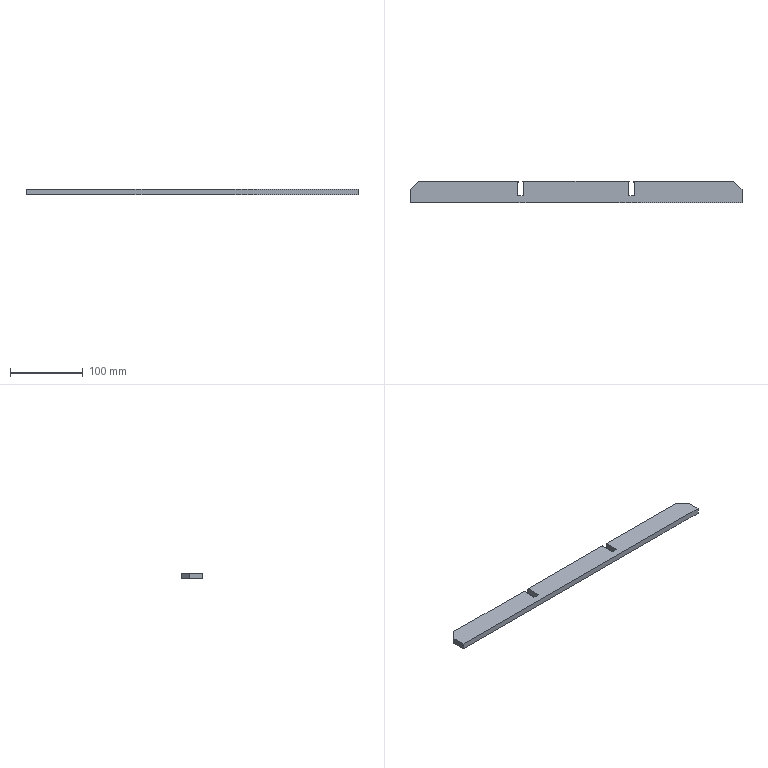Part | SolidWorks | features BaseBody 1 | 1 solid | 18 faces | box 455.8 x 30 x 8 mm | volume 104640 mm3 | plane 18
STEP:
#1=CARTESIAN_POINT('',(73.126,14.398,0.));
#2=VERTEX_POINT('',#1);
#3=CARTESIAN_POINT('',(73.412,15.,8.));
#4=VERTEX_POINT('',#3);
#5=CARTESIAN_POINT('',(73.126,14.398,0.));
#6=DIRECTION('',(0.0356,0.07493,0.9966));
#7=VECTOR('',#6,1000.);
#8=LINE('',#5,#7);
#9=EDGE_CURVE('',#2,#4,#8,.T.);
#10=ORIENTED_EDGE('',*,*,#9,.F.);
#11=CARTESIAN_POINT('',(-73.126,14.398,0.));
#12=VERTEX_POINT('',#11);
#13=CARTESIAN_POINT('',(0.,14.398,0.));
#14=DIRECTION('',(1.,0.,0.));
#15=VECTOR('',#14,1000.);
#16=LINE('',#13,#15);
#17=EDGE_CURVE('',#12,#2,#16,.T.);
#18=ORIENTED_EDGE('',*,*,#17,.F.);
#19=CARTESIAN_POINT('',(-73.412,15.,8.));
#20=VERTEX_POINT('',#19);
#21=CARTESIAN_POINT('',(-73.412,15.,8.));
#22=DIRECTION('',(0.0356,-0.07493,-0.9966));
#23=VECTOR('',#22,1000.);
#24=LINE('',#21,#23);
#25=EDGE_CURVE('',#20,#12,#24,.T.);
#26=ORIENTED_EDGE('',*,*,#25,.F.);
#27=CARTESIAN_POINT('',(0.,15.,8.));
#28=DIRECTION('',(-1.,0.,0.));
#29=VECTOR('',#28,1000.);
#30=LINE('',#27,#29);
#31=EDGE_CURVE('',#4,#20,#30,.T.);
#32=ORIENTED_EDGE('',*,*,#31,.F.);
#33=EDGE_LOOP('',(#10,#18,#26,#32));
#34=FACE_OUTER_BOUND('',#33,.T.);
#35=CARTESIAN_POINT('',(-74.293,15.,8.));
#36=DIRECTION('',(0.,-0.9972,0.07498));
#37=DIRECTION('',(0.,-0.07498,-0.9972));
#38=AXIS2_PLACEMENT_3D('',#35,#36,#37);
#39=PLANE('',#38);
#40=ADVANCED_FACE('',(#34),#39,.F.);
#41=CARTESIAN_POINT('',(71.915,14.956,8.));
#42=VERTEX_POINT('',#41);
#43=CARTESIAN_POINT('',(73.412,15.,8.));
#44=DIRECTION('',(-0.9996,-0.02956,-0.000000001));
#45=VECTOR('',#44,1000.);
#46=LINE('',#43,#45);
#47=EDGE_CURVE('',#4,#42,#46,.T.);
#48=ORIENTED_EDGE('',*,*,#47,.F.);
#49=ORIENTED_EDGE('',*,*,#31,.T.);
#50=CARTESIAN_POINT('',(-71.915,14.956,8.));
#51=VERTEX_POINT('',#50);
#52=CARTESIAN_POINT('',(-71.915,14.956,8.));
#53=DIRECTION('',(-0.9996,0.02956,0.000000001));
#54=VECTOR('',#53,1000.);
#55=LINE('',#52,#54);
#56=EDGE_CURVE('',#51,#20,#55,.T.);
#57=ORIENTED_EDGE('',*,*,#56,.F.);
#58=CARTESIAN_POINT('',(-72.439,-5.092,8.));
#59=VERTEX_POINT('',#58);
#60=CARTESIAN_POINT('',(-72.439,-5.092,8.));
#61=DIRECTION('',(0.02613,0.9997,0.));
#62=VECTOR('',#61,1000.);
#63=LINE('',#60,#62);
#64=EDGE_CURVE('',#59,#51,#63,.T.);
#65=ORIENTED_EDGE('',*,*,#64,.F.);
#66=CARTESIAN_POINT('',(-80.444,-4.856,8.));
#67=VERTEX_POINT('',#66);
#68=CARTESIAN_POINT('',(-80.444,-4.856,8.));
#69=DIRECTION('',(0.9996,-0.02956,0.));
#70=VECTOR('',#69,1000.);
#71=LINE('',#68,#70);
#72=EDGE_CURVE('',#67,#59,#71,.T.);
#73=ORIENTED_EDGE('',*,*,#72,.F.);
#74=CARTESIAN_POINT('',(-79.925,15.,8.));
#75=VERTEX_POINT('',#74);
#76=CARTESIAN_POINT('',(-79.925,15.,8.));
#77=DIRECTION('',(-0.02613,-0.9997,0.));
#78=VECTOR('',#77,1000.);
#79=LINE('',#76,#78);
#80=EDGE_CURVE('',#75,#67,#79,.T.);
#81=ORIENTED_EDGE('',*,*,#80,.F.);
#82=CARTESIAN_POINT('',(-215.9,15.,8.));
#83=VERTEX_POINT('',#82);
#84=CARTESIAN_POINT('',(0.,15.,8.));
#85=DIRECTION('',(1.,0.,0.));
#86=VECTOR('',#85,1000.);
#87=LINE('',#84,#86);
#88=EDGE_CURVE('',#83,#75,#87,.T.);
#89=ORIENTED_EDGE('',*,*,#88,.F.);
#90=CARTESIAN_POINT('',(-227.9,3.,8.));
#91=VERTEX_POINT('',#90);
#92=CARTESIAN_POINT('',(-227.9,3.,8.));
#93=DIRECTION('',(0.7071,0.7071,0.));
#94=VECTOR('',#93,1000.);
#95=LINE('',#92,#94);
#96=EDGE_CURVE('',#91,#83,#95,.T.);
#97=ORIENTED_EDGE('',*,*,#96,.F.);
#98=CARTESIAN_POINT('',(-227.9,-15.,8.));
#99=VERTEX_POINT('',#98);
#100=CARTESIAN_POINT('',(-227.9,0.,8.));
#101=DIRECTION('',(0.,1.,0.));
#102=VECTOR('',#101,1000.);
#103=LINE('',#100,#102);
#104=EDGE_CURVE('',#99,#91,#103,.T.);
#105=ORIENTED_EDGE('',*,*,#104,.F.);
#106=CARTESIAN_POINT('',(227.9,-15.,8.));
#107=VERTEX_POINT('',#106);
#108=CARTESIAN_POINT('',(0.,-15.,8.));
#109=DIRECTION('',(-1.,0.,0.));
#110=VECTOR('',#109,1000.);
#111=LINE('',#108,#110);
#112=EDGE_CURVE('',#107,#99,#111,.T.);
#113=ORIENTED_EDGE('',*,*,#112,.F.);
#114=CARTESIAN_POINT('',(227.9,3.,8.));
#115=VERTEX_POINT('',#114);
#116=CARTESIAN_POINT('',(227.9,0.,8.));
#117=DIRECTION('',(0.,-1.,0.));
#118=VECTOR('',#117,1000.);
#119=LINE('',#116,#118);
#120=EDGE_CURVE('',#115,#107,#119,.T.);
#121=ORIENTED_EDGE('',*,*,#120,.F.);
#122=CARTESIAN_POINT('',(215.9,15.,8.));
#123=VERTEX_POINT('',#122);
#124=CARTESIAN_POINT('',(215.828,15.072,8.));
#125=DIRECTION('',(0.7071,-0.7071,0.));
#126=VECTOR('',#125,1000.);
#127=LINE('',#124,#126);
#128=EDGE_CURVE('',#123,#115,#127,.T.);
#129=ORIENTED_EDGE('',*,*,#128,.F.);
#130=CARTESIAN_POINT('',(79.925,15.,8.));
#131=VERTEX_POINT('',#130);
#132=CARTESIAN_POINT('',(0.,15.,8.));
#133=DIRECTION('',(1.,0.,0.));
#134=VECTOR('',#133,1000.);
#135=LINE('',#132,#134);
#136=EDGE_CURVE('',#131,#123,#135,.T.);
#137=ORIENTED_EDGE('',*,*,#136,.F.);
#138=CARTESIAN_POINT('',(80.444,-4.856,8.));
#139=VERTEX_POINT('',#138);
#140=CARTESIAN_POINT('',(80.444,-4.856,8.));
#141=DIRECTION('',(-0.02613,0.9997,0.));
#142=VECTOR('',#141,1000.);
#143=LINE('',#140,#142);
#144=EDGE_CURVE('',#139,#131,#143,.T.);
#145=ORIENTED_EDGE('',*,*,#144,.F.);
#146=CARTESIAN_POINT('',(72.439,-5.092,8.));
#147=VERTEX_POINT('',#146);
#148=CARTESIAN_POINT('',(72.439,-5.092,8.));
#149=DIRECTION('',(0.9996,0.02956,0.));
#150=VECTOR('',#149,1000.);
#151=LINE('',#148,#150);
#152=EDGE_CURVE('',#147,#139,#151,.T.);
#153=ORIENTED_EDGE('',*,*,#152,.F.);
#154=CARTESIAN_POINT('',(71.915,14.956,8.));
#155=DIRECTION('',(0.02613,-0.9997,0.));
#156=VECTOR('',#155,1000.);
#157=LINE('',#154,#156);
#158=EDGE_CURVE('',#42,#147,#157,.T.);
#159=ORIENTED_EDGE('',*,*,#158,.F.);
#160=EDGE_LOOP('',(#48,#49,#57,#65,#73,#81,#89,#97,#105,#113,#121,#129,#137,#145,#153,#159));
#161=FACE_OUTER_BOUND('',#160,.T.);
#162=CARTESIAN_POINT('',(227.9,-15.,8.));
#163=DIRECTION('',(0.,0.,-1.));
#164=DIRECTION('',(-1.,0.,0.));
#165=AXIS2_PLACEMENT_3D('',#162,#163,#164);
#166=PLANE('',#165);
#167=ADVANCED_FACE('',(#161),#166,.F.);
#168=CARTESIAN_POINT('',(71.56,14.352,0.));
#169=VERTEX_POINT('',#168);
#170=CARTESIAN_POINT('',(73.126,14.398,0.));
#171=DIRECTION('',(-0.9996,-0.02956,0.));
#172=VECTOR('',#171,1000.);
#173=LINE('',#170,#172);
#174=EDGE_CURVE('',#2,#169,#173,.T.);
#175=ORIENTED_EDGE('',*,*,#174,.F.);
#176=ORIENTED_EDGE('',*,*,#9,.T.);
#177=ORIENTED_EDGE('',*,*,#47,.T.);
#178=CARTESIAN_POINT('',(71.56,14.352,0.000000002));
#179=DIRECTION('',(0.04418,0.07516,0.9962));
#180=VECTOR('',#179,1000.);
#181=LINE('',#178,#180);
#182=EDGE_CURVE('',#169,#42,#181,.T.);
#183=ORIENTED_EDGE('',*,*,#182,.F.);
#184=EDGE_LOOP('',(#175,#176,#177,#183));
#185=FACE_OUTER_BOUND('',#184,.T.);
#186=CARTESIAN_POINT('',(71.549,14.348,-0.048));
#187=DIRECTION('',(-0.02948,0.9968,-0.0739));
#188=DIRECTION('',(0.,0.07393,0.9973));
#189=AXIS2_PLACEMENT_3D('',#186,#187,#188);
#190=PLANE('',#189);
#191=ADVANCED_FACE('',(#185),#190,.F.);
#192=CARTESIAN_POINT('',(-71.56,14.352,0.));
#193=VERTEX_POINT('',#192);
#194=CARTESIAN_POINT('',(-71.56,14.352,0.));
#195=DIRECTION('',(-0.9996,0.02956,0.));
#196=VECTOR('',#195,1000.);
#197=LINE('',#194,#196);
#198=EDGE_CURVE('',#193,#12,#197,.T.);
#199=ORIENTED_EDGE('',*,*,#198,.T.);
#200=ORIENTED_EDGE('',*,*,#17,.T.);
#201=ORIENTED_EDGE('',*,*,#174,.T.);
#202=CARTESIAN_POINT('',(72.084,-5.696,0.));
#203=VERTEX_POINT('',#202);
#204=CARTESIAN_POINT('',(71.56,14.352,0.));
#205=DIRECTION('',(0.02613,-0.9997,0.));
#206=VECTOR('',#205,1000.);
#207=LINE('',#204,#206);
#208=EDGE_CURVE('',#169,#203,#207,.T.);
#209=ORIENTED_EDGE('',*,*,#208,.T.);
#210=CARTESIAN_POINT('',(80.089,-5.459,0.));
#211=VERTEX_POINT('',#210);
#212=CARTESIAN_POINT('',(72.084,-5.696,0.));
#213=DIRECTION('',(0.9996,0.02956,0.));
#214=VECTOR('',#213,1000.);
#215=LINE('',#212,#214);
#216=EDGE_CURVE('',#203,#211,#215,.T.);
#217=ORIENTED_EDGE('',*,*,#216,.T.);
#218=CARTESIAN_POINT('',(79.57,14.398,0.));
#219=VERTEX_POINT('',#218);
#220=CARTESIAN_POINT('',(80.089,-5.459,0.));
#221=DIRECTION('',(-0.02613,0.9997,0.));
#222=VECTOR('',#221,1000.);
#223=LINE('',#220,#222);
#224=EDGE_CURVE('',#211,#219,#223,.T.);
#225=ORIENTED_EDGE('',*,*,#224,.T.);
#226=CARTESIAN_POINT('',(216.502,14.398,0.));
#227=VERTEX_POINT('',#226);
#228=CARTESIAN_POINT('',(0.,14.398,0.));
#229=DIRECTION('',(1.,0.,0.));
#230=VECTOR('',#229,1000.);
#231=LINE('',#228,#230);
#232=EDGE_CURVE('',#219,#227,#231,.T.);
#233=ORIENTED_EDGE('',*,*,#232,.T.);
#234=CARTESIAN_POINT('',(227.9,3.,0.));
#235=VERTEX_POINT('',#234);
#236=CARTESIAN_POINT('',(216.502,14.398,0.));
#237=DIRECTION('',(0.7071,-0.7071,0.));
#238=VECTOR('',#237,1000.);
#239=LINE('',#236,#238);
#240=EDGE_CURVE('',#227,#235,#239,.T.);
#241=ORIENTED_EDGE('',*,*,#240,.T.);
#242=CARTESIAN_POINT('',(227.9,-15.,0.));
#243=VERTEX_POINT('',#242);
#244=CARTESIAN_POINT('',(227.9,-0.3008,0.));
#245=DIRECTION('',(0.,-1.,0.));
#246=VECTOR('',#245,1000.);
#247=LINE('',#244,#246);
#248=EDGE_CURVE('',#235,#243,#247,.T.);
#249=ORIENTED_EDGE('',*,*,#248,.T.);
#250=CARTESIAN_POINT('',(-227.9,-15.,0.));
#251=VERTEX_POINT('',#250);
#252=CARTESIAN_POINT('',(0.,-15.,0.));
#253=DIRECTION('',(-1.,0.,0.));
#254=VECTOR('',#253,1000.);
#255=LINE('',#252,#254);
#256=EDGE_CURVE('',#243,#251,#255,.T.);
#257=ORIENTED_EDGE('',*,*,#256,.T.);
#258=CARTESIAN_POINT('',(-227.9,3.,0.));
#259=VERTEX_POINT('',#258);
#260=CARTESIAN_POINT('',(-227.9,-0.3008,0.));
#261=DIRECTION('',(0.,1.,0.));
#262=VECTOR('',#261,1000.);
#263=LINE('',#260,#262);
#264=EDGE_CURVE('',#251,#259,#263,.T.);
#265=ORIENTED_EDGE('',*,*,#264,.T.);
#266=CARTESIAN_POINT('',(-216.502,14.398,0.));
#267=VERTEX_POINT('',#266);
#268=CARTESIAN_POINT('',(-227.9,3.,0.));
#269=DIRECTION('',(0.7071,0.7071,0.));
#270=VECTOR('',#269,1000.);
#271=LINE('',#268,#270);
#272=EDGE_CURVE('',#259,#267,#271,.T.);
#273=ORIENTED_EDGE('',*,*,#272,.T.);
#274=CARTESIAN_POINT('',(-79.57,14.398,0.));
#275=VERTEX_POINT('',#274);
#276=CARTESIAN_POINT('',(0.,14.398,0.));
#277=DIRECTION('',(1.,0.,0.));
#278=VECTOR('',#277,1000.);
#279=LINE('',#276,#278);
#280=EDGE_CURVE('',#267,#275,#279,.T.);
#281=ORIENTED_EDGE('',*,*,#280,.T.);
#282=CARTESIAN_POINT('',(-80.089,-5.459,0.));
#283=VERTEX_POINT('',#282);
#284=CARTESIAN_POINT('',(-79.57,14.398,0.));
#285=DIRECTION('',(-0.02613,-0.9997,0.));
#286=VECTOR('',#285,1000.);
#287=LINE('',#284,#286);
#288=EDGE_CURVE('',#275,#283,#287,.T.);
#289=ORIENTED_EDGE('',*,*,#288,.T.);
#290=CARTESIAN_POINT('',(-72.084,-5.696,0.));
#291=VERTEX_POINT('',#290);
#292=CARTESIAN_POINT('',(-80.089,-5.459,0.));
#293=DIRECTION('',(0.9996,-0.02956,0.));
#294=VECTOR('',#293,1000.);
#295=LINE('',#292,#294);
#296=EDGE_CURVE('',#283,#291,#295,.T.);
#297=ORIENTED_EDGE('',*,*,#296,.T.);
#298=CARTESIAN_POINT('',(-72.084,-5.696,0.));
#299=DIRECTION('',(0.02613,0.9997,0.));
#300=VECTOR('',#299,1000.);
#301=LINE('',#298,#300);
#302=EDGE_CURVE('',#291,#193,#301,.T.);
#303=ORIENTED_EDGE('',*,*,#302,.T.);
#304=EDGE_LOOP('',(#199,#200,#201,#209,#217,#225,#233,#241,#249,#257,#265,#273,#281,#289,#297,#303));
#305=FACE_OUTER_BOUND('',#304,.T.);
#306=CARTESIAN_POINT('',(227.9,-15.,0.));
#307=DIRECTION('',(0.,0.,-1.));
#308=DIRECTION('',(-1.,0.,0.));
#309=AXIS2_PLACEMENT_3D('',#306,#307,#308);
#310=PLANE('',#309);
#311=ADVANCED_FACE('',(#305),#310,.T.);
#312=ORIENTED_EDGE('',*,*,#198,.F.);
#313=CARTESIAN_POINT('',(-71.915,14.956,8.));
#314=DIRECTION('',(0.04418,-0.07516,-0.9962));
#315=VECTOR('',#314,1000.);
#316=LINE('',#313,#315);
#317=EDGE_CURVE('',#51,#193,#316,.T.);
#318=ORIENTED_EDGE('',*,*,#317,.F.);
#319=ORIENTED_EDGE('',*,*,#56,.T.);
#320=ORIENTED_EDGE('',*,*,#25,.T.);
#321=EDGE_LOOP('',(#312,#318,#319,#320));
#322=FACE_OUTER_BOUND('',#321,.T.);
#323=CARTESIAN_POINT('',(-73.423,14.403,-0.05209));
#324=DIRECTION('',(0.02948,0.9968,-0.0739));
#325=DIRECTION('',(0.,0.07393,0.9973));
#326=AXIS2_PLACEMENT_3D('',#323,#324,#325);
#327=PLANE('',#326);
#328=ADVANCED_FACE('',(#322),#327,.F.);
#329=ORIENTED_EDGE('',*,*,#208,.F.);
#330=ORIENTED_EDGE('',*,*,#182,.T.);
#331=ORIENTED_EDGE('',*,*,#158,.T.);
#332=CARTESIAN_POINT('',(72.084,-5.696,0.000000004));
#333=DIRECTION('',(0.04418,0.07516,0.9962));
#334=VECTOR('',#333,1000.);
#335=LINE('',#332,#334);
#336=EDGE_CURVE('',#203,#147,#335,.T.);
#337=ORIENTED_EDGE('',*,*,#336,.F.);
#338=EDGE_LOOP('',(#329,#330,#331,#337));
#339=FACE_OUTER_BOUND('',#338,.T.);
#340=CARTESIAN_POINT('',(72.084,-5.82,-0.07251));
#341=DIRECTION('',(-0.9986,-0.0261,0.04626));
#342=DIRECTION('',(0.04627,0.,0.9989));
#343=AXIS2_PLACEMENT_3D('',#340,#341,#342);
#344=PLANE('',#343);
#345=ADVANCED_FACE('',(#339),#344,.F.);
#346=ORIENTED_EDGE('',*,*,#302,.F.);
#347=CARTESIAN_POINT('',(-72.439,-5.092,8.));
#348=DIRECTION('',(0.04418,-0.07516,-0.9962));
#349=VECTOR('',#348,1000.);
#350=LINE('',#347,#349);
#351=EDGE_CURVE('',#59,#291,#350,.T.);
#352=ORIENTED_EDGE('',*,*,#351,.F.);
#353=ORIENTED_EDGE('',*,*,#64,.T.);
#354=ORIENTED_EDGE('',*,*,#317,.T.);
#355=EDGE_LOOP('',(#346,#352,#353,#354));
#356=FACE_OUTER_BOUND('',#355,.T.);
#357=CARTESIAN_POINT('',(-72.46,-5.82,8.047));
#358=DIRECTION('',(0.9986,-0.0261,0.04626));
#359=DIRECTION('',(0.04627,0.,-0.9989));
#360=AXIS2_PLACEMENT_3D('',#357,#358,#359);
#361=PLANE('',#360);
#362=ADVANCED_FACE('',(#356),#361,.F.);
#363=ORIENTED_EDGE('',*,*,#296,.F.);
#364=CARTESIAN_POINT('',(-80.444,-4.856,8.));
#365=DIRECTION('',(0.04418,-0.07516,-0.9962));
#366=VECTOR('',#365,1000.);
#367=LINE('',#364,#366);
#368=EDGE_CURVE('',#67,#283,#367,.T.);
#369=ORIENTED_EDGE('',*,*,#368,.F.);
#370=ORIENTED_EDGE('',*,*,#72,.T.);
#371=ORIENTED_EDGE('',*,*,#351,.T.);
#372=EDGE_LOOP('',(#363,#369,#370,#371));
#373=FACE_OUTER_BOUND('',#372,.T.);
#374=CARTESIAN_POINT('',(-80.494,-4.851,8.048));
#375=DIRECTION('',(-0.02948,-0.9968,0.0739));
#376=DIRECTION('',(0.,-0.07393,-0.9973));
#377=AXIS2_PLACEMENT_3D('',#374,#375,#376);
#378=PLANE('',#377);
#379=ADVANCED_FACE('',(#373),#378,.F.);
#380=ORIENTED_EDGE('',*,*,#288,.F.);
#381=CARTESIAN_POINT('',(-79.925,15.,8.));
#382=DIRECTION('',(0.04419,-0.07491,-0.9962));
#383=VECTOR('',#382,1000.);
#384=LINE('',#381,#383);
#385=EDGE_CURVE('',#75,#275,#384,.T.);
#386=ORIENTED_EDGE('',*,*,#385,.F.);
#387=ORIENTED_EDGE('',*,*,#80,.T.);
#388=ORIENTED_EDGE('',*,*,#368,.T.);
#389=EDGE_LOOP('',(#380,#386,#387,#388));
#390=FACE_OUTER_BOUND('',#389,.T.);
#391=CARTESIAN_POINT('',(-80.089,-5.582,-0.07228));
#392=DIRECTION('',(-0.9986,0.0261,-0.04626));
#393=DIRECTION('',(-0.04627,0.,0.9989));
#394=AXIS2_PLACEMENT_3D('',#391,#392,#393);
#395=PLANE('',#394);
#396=ADVANCED_FACE('',(#390),#395,.F.);
#397=ORIENTED_EDGE('',*,*,#385,.T.);
#398=ORIENTED_EDGE('',*,*,#280,.F.);
#399=CARTESIAN_POINT('',(-215.9,15.,8.));
#400=DIRECTION('',(-0.07477,-0.07477,-0.9944));
#401=VECTOR('',#400,1000.);
#402=LINE('',#399,#401);
#403=EDGE_CURVE('',#83,#267,#402,.T.);
#404=ORIENTED_EDGE('',*,*,#403,.F.);
#405=ORIENTED_EDGE('',*,*,#88,.T.);
#406=EDGE_LOOP('',(#397,#398,#404,#405));
#407=FACE_OUTER_BOUND('',#406,.T.);
#408=CARTESIAN_POINT('',(-217.323,15.,8.));
#409=DIRECTION('',(0.,-0.9972,0.07498));
#410=DIRECTION('',(0.,-0.07498,-0.9972));
#411=AXIS2_PLACEMENT_3D('',#408,#409,#410);
#412=PLANE('',#411);
#413=ADVANCED_FACE('',(#407),#412,.F.);
#414=ORIENTED_EDGE('',*,*,#403,.T.);
#415=ORIENTED_EDGE('',*,*,#272,.F.);
#416=CARTESIAN_POINT('',(-227.9,3.,4.));
#417=DIRECTION('',(0.,0.,-1.));
#418=VECTOR('',#417,1000.);
#419=LINE('',#416,#418);
#420=EDGE_CURVE('',#91,#259,#419,.T.);
#421=ORIENTED_EDGE('',*,*,#420,.F.);
#422=ORIENTED_EDGE('',*,*,#96,.T.);
#423=EDGE_LOOP('',(#414,#415,#421,#422));
#424=FACE_OUTER_BOUND('',#423,.T.);
#425=CARTESIAN_POINT('',(-227.9,3.,0.));
#426=DIRECTION('',(0.7071,-0.7071,0.));
#427=DIRECTION('',(0.7071,0.7071,0.));
#428=AXIS2_PLACEMENT_3D('',#425,#426,#427);
#429=PLANE('',#428);
#430=ADVANCED_FACE('',(#424),#429,.F.);
#431=CARTESIAN_POINT('',(-227.9,-15.,4.));
#432=DIRECTION('',(0.,0.,-1.));
#433=VECTOR('',#432,1000.);
#434=LINE('',#431,#433);
#435=EDGE_CURVE('',#99,#251,#434,.T.);
#436=ORIENTED_EDGE('',*,*,#435,.F.);
#437=ORIENTED_EDGE('',*,*,#104,.T.);
#438=ORIENTED_EDGE('',*,*,#420,.T.);
#439=ORIENTED_EDGE('',*,*,#264,.F.);
#440=EDGE_LOOP('',(#436,#437,#438,#439));
#441=FACE_OUTER_BOUND('',#440,.T.);
#442=CARTESIAN_POINT('',(-227.9,-15.,0.));
#443=DIRECTION('',(1.,0.,0.));
#444=DIRECTION('',(0.,1.,0.));
#445=AXIS2_PLACEMENT_3D('',#442,#443,#444);
#446=PLANE('',#445);
#447=ADVANCED_FACE('',(#441),#446,.F.);
#448=CARTESIAN_POINT('',(227.9,-15.,4.));
#449=DIRECTION('',(0.,0.,-1.));
#450=VECTOR('',#449,1000.);
#451=LINE('',#448,#450);
#452=EDGE_CURVE('',#107,#243,#451,.T.);
#453=ORIENTED_EDGE('',*,*,#452,.F.);
#454=ORIENTED_EDGE('',*,*,#112,.T.);
#455=ORIENTED_EDGE('',*,*,#435,.T.);
#456=ORIENTED_EDGE('',*,*,#256,.F.);
#457=EDGE_LOOP('',(#453,#454,#455,#456));
#458=FACE_OUTER_BOUND('',#457,.T.);
#459=CARTESIAN_POINT('',(227.9,-15.,0.));
#460=DIRECTION('',(0.,1.,0.));
#461=DIRECTION('',(-1.,0.,0.));
#462=AXIS2_PLACEMENT_3D('',#459,#460,#461);
#463=PLANE('',#462);
#464=ADVANCED_FACE('',(#458),#463,.F.);
#465=CARTESIAN_POINT('',(227.9,3.,4.));
#466=DIRECTION('',(0.,0.,-1.));
#467=VECTOR('',#466,1000.);
#468=LINE('',#465,#467);
#469=EDGE_CURVE('',#115,#235,#468,.T.);
#470=ORIENTED_EDGE('',*,*,#469,.F.);
#471=ORIENTED_EDGE('',*,*,#120,.T.);
#472=ORIENTED_EDGE('',*,*,#452,.T.);
#473=ORIENTED_EDGE('',*,*,#248,.F.);
#474=EDGE_LOOP('',(#470,#471,#472,#473));
#475=FACE_OUTER_BOUND('',#474,.T.);
#476=CARTESIAN_POINT('',(227.9,-15.,0.));
#477=DIRECTION('',(-1.,0.,0.));
#478=DIRECTION('',(0.,0.,1.));
#479=AXIS2_PLACEMENT_3D('',#476,#477,#478);
#480=PLANE('',#479);
#481=ADVANCED_FACE('',(#475),#480,.F.);
#482=CARTESIAN_POINT('',(215.9,15.,8.));
#483=DIRECTION('',(0.07477,-0.07477,-0.9944));
#484=VECTOR('',#483,1000.);
#485=LINE('',#482,#484);
#486=EDGE_CURVE('',#123,#227,#485,.T.);
#487=ORIENTED_EDGE('',*,*,#486,.F.);
#488=ORIENTED_EDGE('',*,*,#128,.T.);
#489=ORIENTED_EDGE('',*,*,#469,.T.);
#490=ORIENTED_EDGE('',*,*,#240,.F.);
#491=EDGE_LOOP('',(#487,#488,#489,#490));
#492=FACE_OUTER_BOUND('',#491,.T.);
#493=CARTESIAN_POINT('',(215.828,15.072,0.));
#494=DIRECTION('',(-0.7071,-0.7071,0.));
#495=DIRECTION('',(0.7071,-0.7071,0.));
#496=AXIS2_PLACEMENT_3D('',#493,#494,#495);
#497=PLANE('',#496);
#498=ADVANCED_FACE('',(#492),#497,.F.);
#499=CARTESIAN_POINT('',(79.925,15.,8.));
#500=DIRECTION('',(-0.04419,-0.07491,-0.9962));
#501=VECTOR('',#500,1000.);
#502=LINE('',#499,#501);
#503=EDGE_CURVE('',#131,#219,#502,.T.);
#504=ORIENTED_EDGE('',*,*,#503,.F.);
#505=ORIENTED_EDGE('',*,*,#136,.T.);
#506=ORIENTED_EDGE('',*,*,#486,.T.);
#507=ORIENTED_EDGE('',*,*,#232,.F.);
#508=EDGE_LOOP('',(#504,#505,#506,#507));
#509=FACE_OUTER_BOUND('',#508,.T.);
#510=CARTESIAN_POINT('',(78.749,15.,8.));
#511=DIRECTION('',(0.,-0.9972,0.07498));
#512=DIRECTION('',(0.,-0.07498,-0.9972));
#513=AXIS2_PLACEMENT_3D('',#510,#511,#512);
#514=PLANE('',#513);
#515=ADVANCED_FACE('',(#509),#514,.F.);
#516=ORIENTED_EDGE('',*,*,#224,.F.);
#517=CARTESIAN_POINT('',(80.444,-4.856,8.));
#518=DIRECTION('',(-0.04418,-0.07516,-0.9962));
#519=VECTOR('',#518,1000.);
#520=LINE('',#517,#519);
#521=EDGE_CURVE('',#139,#211,#520,.T.);
#522=ORIENTED_EDGE('',*,*,#521,.F.);
#523=ORIENTED_EDGE('',*,*,#144,.T.);
#524=ORIENTED_EDGE('',*,*,#503,.T.);
#525=EDGE_LOOP('',(#516,#522,#523,#524));
#526=FACE_OUTER_BOUND('',#525,.T.);
#527=CARTESIAN_POINT('',(80.465,-5.582,8.047));
#528=DIRECTION('',(0.9986,0.0261,-0.04626));
#529=DIRECTION('',(-0.04627,0.,-0.9989));
#530=AXIS2_PLACEMENT_3D('',#527,#528,#529);
#531=PLANE('',#530);
#532=ADVANCED_FACE('',(#526),#531,.F.);
#533=ORIENTED_EDGE('',*,*,#216,.F.);
#534=ORIENTED_EDGE('',*,*,#336,.T.);
#535=ORIENTED_EDGE('',*,*,#152,.T.);
#536=ORIENTED_EDGE('',*,*,#521,.T.);
#537=EDGE_LOOP('',(#533,#534,#535,#536));
#538=FACE_OUTER_BOUND('',#537,.T.);
#539=CARTESIAN_POINT('',(72.034,-5.099,8.066));
#540=DIRECTION('',(0.02948,-0.9968,0.0739));
#541=DIRECTION('',(0.,-0.07393,-0.9973));
#542=AXIS2_PLACEMENT_3D('',#539,#540,#541);
#543=PLANE('',#542);
#544=ADVANCED_FACE('',(#538),#543,.F.);
#545=CLOSED_SHELL('',(#40,#167,#191,#311,#328,#345,#362,#379,#396,#413,#430,#447,#464,#481,#498,#515,#532,#544));
#546=MANIFOLD_SOLID_BREP('',#545);
#547=CARTESIAN_POINT('',(0.,0.,0.));
#548=DIRECTION('',(0.,0.,1.));
#549=DIRECTION('',(1.,0.,0.));
#550=AXIS2_PLACEMENT_3D('',#547,#548,#549);
#551=(LENGTH_UNIT()NAMED_UNIT(*)SI_UNIT(.MILLI.,.METRE.));
#552=UNCERTAINTY_MEASURE_WITH_UNIT(LENGTH_MEASURE(0.00001),#551,'','');
#553=(NAMED_UNIT(*)PLANE_ANGLE_UNIT()SI_UNIT($,.RADIAN.));
#554=(NAMED_UNIT(*)SI_UNIT($,.STERADIAN.)SOLID_ANGLE_UNIT());
#555=(GEOMETRIC_REPRESENTATION_CONTEXT(3)GLOBAL_UNCERTAINTY_ASSIGNED_CONTEXT((#552))GLOBAL_UNIT_ASSIGNED_CONTEXT((#551,#553,#554))REPRESENTATION_CONTEXT('',''));
#556=ADVANCED_BREP_SHAPE_REPRESENTATION('',(#546,#550),#555);